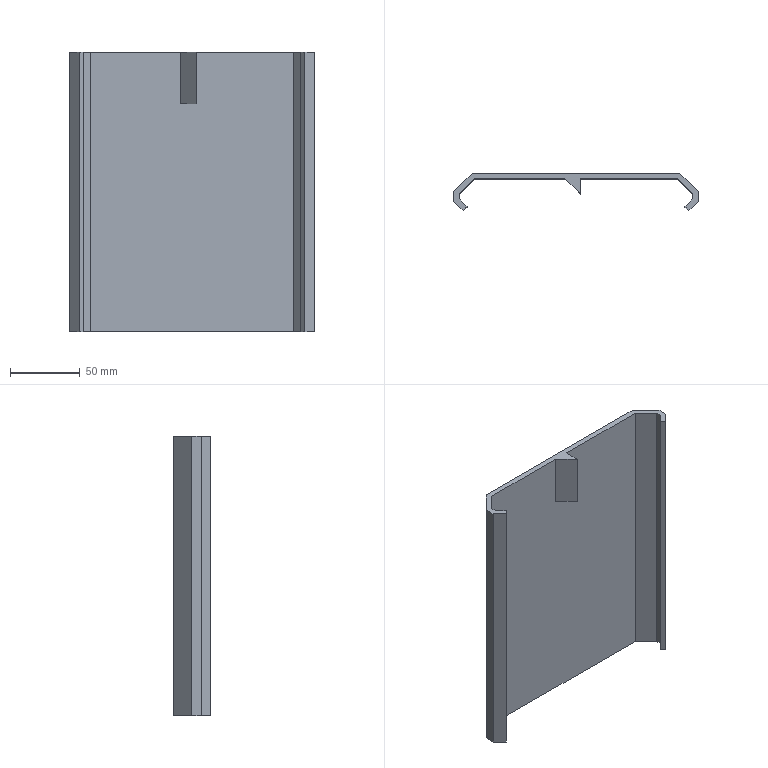Part | SolidWorks | features ExtruThin 1, ICE 1 | 1 solid | 21 faces | box 175 x 26.828 x 200 mm | volume 169317 mm3 | plane 21
STEP:
#1=CARTESIAN_POINT('',(83.5,37.5,0.));
#2=VERTEX_POINT('',#1);
#3=CARTESIAN_POINT('',(78.,32.,0.));
#4=VERTEX_POINT('',#3);
#5=CARTESIAN_POINT('',(83.5,37.5,0.));
#6=DIRECTION('',(-0.7071,-0.7071,0.));
#7=VECTOR('',#6,1000.);
#8=LINE('',#5,#7);
#9=EDGE_CURVE('',#2,#4,#8,.T.);
#10=ORIENTED_EDGE('',*,*,#9,.F.);
#11=CARTESIAN_POINT('',(83.5,37.5,-200.));
#12=VERTEX_POINT('',#11);
#13=CARTESIAN_POINT('',(83.5,37.5,-200.));
#14=DIRECTION('',(0.,0.,1.));
#15=VECTOR('',#14,1000.);
#16=LINE('',#13,#15);
#17=EDGE_CURVE('',#12,#2,#16,.T.);
#18=ORIENTED_EDGE('',*,*,#17,.F.);
#19=CARTESIAN_POINT('',(78.,32.,-200.));
#20=VERTEX_POINT('',#19);
#21=CARTESIAN_POINT('',(83.5,37.5,-200.));
#22=DIRECTION('',(-0.7071,-0.7071,0.));
#23=VECTOR('',#22,1000.);
#24=LINE('',#21,#23);
#25=EDGE_CURVE('',#12,#20,#24,.T.);
#26=ORIENTED_EDGE('',*,*,#25,.T.);
#27=CARTESIAN_POINT('',(78.,32.,-200.));
#28=DIRECTION('',(0.,0.,1.));
#29=VECTOR('',#28,1000.);
#30=LINE('',#27,#29);
#31=EDGE_CURVE('',#20,#4,#30,.T.);
#32=ORIENTED_EDGE('',*,*,#31,.T.);
#33=EDGE_LOOP('',(#10,#18,#26,#32));
#34=FACE_OUTER_BOUND('',#33,.T.);
#35=CARTESIAN_POINT('',(83.5,37.5,-200.));
#36=DIRECTION('',(-0.7071,0.7071,0.));
#37=DIRECTION('',(-0.7071,-0.7071,0.));
#38=AXIS2_PLACEMENT_3D('',#35,#36,#37);
#39=PLANE('',#38);
#40=ADVANCED_FACE('',(#34),#39,.T.);
#41=CARTESIAN_POINT('',(83.5,41.207,0.));
#42=VERTEX_POINT('',#41);
#43=CARTESIAN_POINT('',(83.5,41.207,0.));
#44=DIRECTION('',(0.,-1.,0.));
#45=VECTOR('',#44,1000.);
#46=LINE('',#43,#45);
#47=EDGE_CURVE('',#42,#2,#46,.T.);
#48=ORIENTED_EDGE('',*,*,#47,.F.);
#49=CARTESIAN_POINT('',(83.5,41.207,-200.));
#50=VERTEX_POINT('',#49);
#51=CARTESIAN_POINT('',(83.5,41.207,-200.));
#52=DIRECTION('',(0.,0.,1.));
#53=VECTOR('',#52,1000.);
#54=LINE('',#51,#53);
#55=EDGE_CURVE('',#50,#42,#54,.T.);
#56=ORIENTED_EDGE('',*,*,#55,.F.);
#57=CARTESIAN_POINT('',(83.5,41.207,-200.));
#58=DIRECTION('',(0.,-1.,0.));
#59=VECTOR('',#58,1000.);
#60=LINE('',#57,#59);
#61=EDGE_CURVE('',#50,#12,#60,.T.);
#62=ORIENTED_EDGE('',*,*,#61,.T.);
#63=ORIENTED_EDGE('',*,*,#17,.T.);
#64=EDGE_LOOP('',(#48,#56,#62,#63));
#65=FACE_OUTER_BOUND('',#64,.T.);
#66=CARTESIAN_POINT('',(83.5,41.207,-200.));
#67=DIRECTION('',(-1.,0.,0.));
#68=DIRECTION('',(0.,0.,1.));
#69=AXIS2_PLACEMENT_3D('',#66,#67,#68);
#70=PLANE('',#69);
#71=ADVANCED_FACE('',(#65),#70,.T.);
#72=CARTESIAN_POINT('',(72.707,52.,0.));
#73=VERTEX_POINT('',#72);
#74=CARTESIAN_POINT('',(72.707,52.,0.));
#75=DIRECTION('',(0.7071,-0.7071,0.));
#76=VECTOR('',#75,1000.);
#77=LINE('',#74,#76);
#78=EDGE_CURVE('',#73,#42,#77,.T.);
#79=ORIENTED_EDGE('',*,*,#78,.F.);
#80=CARTESIAN_POINT('',(72.707,52.,-200.));
#81=VERTEX_POINT('',#80);
#82=CARTESIAN_POINT('',(72.707,52.,-200.));
#83=DIRECTION('',(0.,0.,1.));
#84=VECTOR('',#83,1000.);
#85=LINE('',#82,#84);
#86=EDGE_CURVE('',#81,#73,#85,.T.);
#87=ORIENTED_EDGE('',*,*,#86,.F.);
#88=CARTESIAN_POINT('',(72.707,52.,-200.));
#89=DIRECTION('',(0.7071,-0.7071,0.));
#90=VECTOR('',#89,1000.);
#91=LINE('',#88,#90);
#92=EDGE_CURVE('',#81,#50,#91,.T.);
#93=ORIENTED_EDGE('',*,*,#92,.T.);
#94=ORIENTED_EDGE('',*,*,#55,.T.);
#95=EDGE_LOOP('',(#79,#87,#93,#94));
#96=FACE_OUTER_BOUND('',#95,.T.);
#97=CARTESIAN_POINT('',(72.707,52.,-200.));
#98=DIRECTION('',(-0.7071,-0.7071,0.));
#99=DIRECTION('',(0.7071,-0.7071,0.));
#100=AXIS2_PLACEMENT_3D('',#97,#98,#99);
#101=PLANE('',#100);
#102=ADVANCED_FACE('',(#96),#101,.T.);
#103=CARTESIAN_POINT('',(-7.99,52.,-37.));
#104=VERTEX_POINT('',#103);
#105=CARTESIAN_POINT('',(-7.99,52.,0.));
#106=VERTEX_POINT('',#105);
#107=CARTESIAN_POINT('',(-7.99,52.,-37.));
#108=DIRECTION('',(0.,0.,1.));
#109=VECTOR('',#108,1000.);
#110=LINE('',#107,#109);
#111=EDGE_CURVE('',#104,#106,#110,.T.);
#112=ORIENTED_EDGE('',*,*,#111,.T.);
#113=CARTESIAN_POINT('',(-72.707,52.,0.));
#114=VERTEX_POINT('',#113);
#115=CARTESIAN_POINT('',(72.707,52.,0.));
#116=DIRECTION('',(1.,0.,0.));
#117=VECTOR('',#116,1000.);
#118=LINE('',#115,#117);
#119=EDGE_CURVE('',#114,#106,#118,.T.);
#120=ORIENTED_EDGE('',*,*,#119,.F.);
#121=CARTESIAN_POINT('',(-72.707,52.,-200.));
#122=VERTEX_POINT('',#121);
#123=CARTESIAN_POINT('',(-72.707,52.,-200.));
#124=DIRECTION('',(0.,0.,1.));
#125=VECTOR('',#124,1000.);
#126=LINE('',#123,#125);
#127=EDGE_CURVE('',#122,#114,#126,.T.);
#128=ORIENTED_EDGE('',*,*,#127,.F.);
#129=CARTESIAN_POINT('',(72.707,52.,-200.));
#130=DIRECTION('',(1.,0.,0.));
#131=VECTOR('',#130,1000.);
#132=LINE('',#129,#131);
#133=EDGE_CURVE('',#122,#81,#132,.T.);
#134=ORIENTED_EDGE('',*,*,#133,.T.);
#135=ORIENTED_EDGE('',*,*,#86,.T.);
#136=CARTESIAN_POINT('',(3.,52.,0.));
#137=VERTEX_POINT('',#136);
#138=CARTESIAN_POINT('',(72.707,52.,0.));
#139=DIRECTION('',(1.,0.,0.));
#140=VECTOR('',#139,1000.);
#141=LINE('',#138,#140);
#142=EDGE_CURVE('',#137,#73,#141,.T.);
#143=ORIENTED_EDGE('',*,*,#142,.F.);
#144=CARTESIAN_POINT('',(3.,52.,-37.));
#145=VERTEX_POINT('',#144);
#146=CARTESIAN_POINT('',(3.,52.,-37.));
#147=DIRECTION('',(0.,0.,1.));
#148=VECTOR('',#147,1000.);
#149=LINE('',#146,#148);
#150=EDGE_CURVE('',#145,#137,#149,.T.);
#151=ORIENTED_EDGE('',*,*,#150,.F.);
#152=CARTESIAN_POINT('',(-7.99,52.,-37.));
#153=DIRECTION('',(-1.,0.,0.));
#154=VECTOR('',#153,1000.);
#155=LINE('',#152,#154);
#156=EDGE_CURVE('',#145,#104,#155,.T.);
#157=ORIENTED_EDGE('',*,*,#156,.T.);
#158=EDGE_LOOP('',(#112,#120,#128,#134,#135,#143,#151,#157));
#159=FACE_OUTER_BOUND('',#158,.T.);
#160=CARTESIAN_POINT('',(72.707,52.,-200.));
#161=DIRECTION('',(0.,-1.,0.));
#162=DIRECTION('',(0.,0.,-1.));
#163=AXIS2_PLACEMENT_3D('',#160,#161,#162);
#164=PLANE('',#163);
#165=ADVANCED_FACE('',(#159),#164,.T.);
#166=CARTESIAN_POINT('',(-83.5,41.207,0.));
#167=VERTEX_POINT('',#166);
#168=CARTESIAN_POINT('',(-72.707,52.,0.));
#169=DIRECTION('',(0.7071,0.7071,0.));
#170=VECTOR('',#169,1000.);
#171=LINE('',#168,#170);
#172=EDGE_CURVE('',#167,#114,#171,.T.);
#173=ORIENTED_EDGE('',*,*,#172,.F.);
#174=CARTESIAN_POINT('',(-83.5,41.207,-200.));
#175=VERTEX_POINT('',#174);
#176=CARTESIAN_POINT('',(-83.5,41.207,-200.));
#177=DIRECTION('',(0.,0.,1.));
#178=VECTOR('',#177,1000.);
#179=LINE('',#176,#178);
#180=EDGE_CURVE('',#175,#167,#179,.T.);
#181=ORIENTED_EDGE('',*,*,#180,.F.);
#182=CARTESIAN_POINT('',(-72.707,52.,-200.));
#183=DIRECTION('',(0.7071,0.7071,0.));
#184=VECTOR('',#183,1000.);
#185=LINE('',#182,#184);
#186=EDGE_CURVE('',#175,#122,#185,.T.);
#187=ORIENTED_EDGE('',*,*,#186,.T.);
#188=ORIENTED_EDGE('',*,*,#127,.T.);
#189=EDGE_LOOP('',(#173,#181,#187,#188));
#190=FACE_OUTER_BOUND('',#189,.T.);
#191=CARTESIAN_POINT('',(-72.707,52.,-200.));
#192=DIRECTION('',(0.7071,-0.7071,0.));
#193=DIRECTION('',(0.7071,0.7071,0.));
#194=AXIS2_PLACEMENT_3D('',#191,#192,#193);
#195=PLANE('',#194);
#196=ADVANCED_FACE('',(#190),#195,.T.);
#197=CARTESIAN_POINT('',(-83.5,37.5,0.));
#198=VERTEX_POINT('',#197);
#199=CARTESIAN_POINT('',(-83.5,41.207,0.));
#200=DIRECTION('',(0.,1.,0.));
#201=VECTOR('',#200,1000.);
#202=LINE('',#199,#201);
#203=EDGE_CURVE('',#198,#167,#202,.T.);
#204=ORIENTED_EDGE('',*,*,#203,.F.);
#205=CARTESIAN_POINT('',(-83.5,37.5,-200.));
#206=VERTEX_POINT('',#205);
#207=CARTESIAN_POINT('',(-83.5,37.5,-200.));
#208=DIRECTION('',(0.,0.,1.));
#209=VECTOR('',#208,1000.);
#210=LINE('',#207,#209);
#211=EDGE_CURVE('',#206,#198,#210,.T.);
#212=ORIENTED_EDGE('',*,*,#211,.F.);
#213=CARTESIAN_POINT('',(-83.5,41.207,-200.));
#214=DIRECTION('',(0.,1.,0.));
#215=VECTOR('',#214,1000.);
#216=LINE('',#213,#215);
#217=EDGE_CURVE('',#206,#175,#216,.T.);
#218=ORIENTED_EDGE('',*,*,#217,.T.);
#219=ORIENTED_EDGE('',*,*,#180,.T.);
#220=EDGE_LOOP('',(#204,#212,#218,#219));
#221=FACE_OUTER_BOUND('',#220,.T.);
#222=CARTESIAN_POINT('',(-83.5,41.207,-200.));
#223=DIRECTION('',(1.,0.,0.));
#224=DIRECTION('',(0.,0.,-1.));
#225=AXIS2_PLACEMENT_3D('',#222,#223,#224);
#226=PLANE('',#225);
#227=ADVANCED_FACE('',(#221),#226,.T.);
#228=CARTESIAN_POINT('',(-78.,32.,0.));
#229=VERTEX_POINT('',#228);
#230=CARTESIAN_POINT('',(-83.5,37.5,0.));
#231=DIRECTION('',(-0.7071,0.7071,0.));
#232=VECTOR('',#231,1000.);
#233=LINE('',#230,#232);
#234=EDGE_CURVE('',#229,#198,#233,.T.);
#235=ORIENTED_EDGE('',*,*,#234,.F.);
#236=CARTESIAN_POINT('',(-78.,32.,-200.));
#237=VERTEX_POINT('',#236);
#238=CARTESIAN_POINT('',(-78.,32.,-200.));
#239=DIRECTION('',(0.,0.,1.));
#240=VECTOR('',#239,1000.);
#241=LINE('',#238,#240);
#242=EDGE_CURVE('',#237,#229,#241,.T.);
#243=ORIENTED_EDGE('',*,*,#242,.F.);
#244=CARTESIAN_POINT('',(-83.5,37.5,-200.));
#245=DIRECTION('',(-0.7071,0.7071,0.));
#246=VECTOR('',#245,1000.);
#247=LINE('',#244,#246);
#248=EDGE_CURVE('',#237,#206,#247,.T.);
#249=ORIENTED_EDGE('',*,*,#248,.T.);
#250=ORIENTED_EDGE('',*,*,#211,.T.);
#251=EDGE_LOOP('',(#235,#243,#249,#250));
#252=FACE_OUTER_BOUND('',#251,.T.);
#253=CARTESIAN_POINT('',(-83.5,37.5,-200.));
#254=DIRECTION('',(0.7071,0.7071,0.));
#255=DIRECTION('',(-0.7071,0.7071,0.));
#256=AXIS2_PLACEMENT_3D('',#253,#254,#255);
#257=PLANE('',#256);
#258=ADVANCED_FACE('',(#252),#257,.T.);
#259=CARTESIAN_POINT('',(-80.828,29.172,0.));
#260=VERTEX_POINT('',#259);
#261=CARTESIAN_POINT('',(-78.,32.,0.));
#262=DIRECTION('',(-0.7071,-0.7071,0.));
#263=VECTOR('',#262,1000.);
#264=LINE('',#261,#263);
#265=EDGE_CURVE('',#229,#260,#264,.T.);
#266=ORIENTED_EDGE('',*,*,#265,.T.);
#267=CARTESIAN_POINT('',(-80.828,29.172,-200.));
#268=VERTEX_POINT('',#267);
#269=CARTESIAN_POINT('',(-80.828,29.172,-200.));
#270=DIRECTION('',(0.,0.,1.));
#271=VECTOR('',#270,1000.);
#272=LINE('',#269,#271);
#273=EDGE_CURVE('',#268,#260,#272,.T.);
#274=ORIENTED_EDGE('',*,*,#273,.F.);
#275=CARTESIAN_POINT('',(-78.,32.,-200.));
#276=DIRECTION('',(-0.7071,-0.7071,0.));
#277=VECTOR('',#276,1000.);
#278=LINE('',#275,#277);
#279=EDGE_CURVE('',#237,#268,#278,.T.);
#280=ORIENTED_EDGE('',*,*,#279,.F.);
#281=ORIENTED_EDGE('',*,*,#242,.T.);
#282=EDGE_LOOP('',(#266,#274,#280,#281));
#283=FACE_OUTER_BOUND('',#282,.T.);
#284=CARTESIAN_POINT('',(-78.,32.,-200.));
#285=DIRECTION('',(-0.7071,0.7071,0.));
#286=DIRECTION('',(-0.7071,-0.7071,0.));
#287=AXIS2_PLACEMENT_3D('',#284,#285,#286);
#288=PLANE('',#287);
#289=ADVANCED_FACE('',(#283),#288,.F.);
#290=CARTESIAN_POINT('',(-87.5,35.843,0.));
#291=VERTEX_POINT('',#290);
#292=CARTESIAN_POINT('',(-86.328,34.672,0.));
#293=DIRECTION('',(-0.7071,0.7071,0.));
#294=VECTOR('',#293,1000.);
#295=LINE('',#292,#294);
#296=EDGE_CURVE('',#260,#291,#295,.T.);
#297=ORIENTED_EDGE('',*,*,#296,.T.);
#298=CARTESIAN_POINT('',(-87.5,35.843,-200.));
#299=VERTEX_POINT('',#298);
#300=CARTESIAN_POINT('',(-87.5,35.843,-200.));
#301=DIRECTION('',(0.,0.,1.));
#302=VECTOR('',#301,1000.);
#303=LINE('',#300,#302);
#304=EDGE_CURVE('',#299,#291,#303,.T.);
#305=ORIENTED_EDGE('',*,*,#304,.F.);
#306=CARTESIAN_POINT('',(-86.328,34.672,-200.));
#307=DIRECTION('',(-0.7071,0.7071,0.));
#308=VECTOR('',#307,1000.);
#309=LINE('',#306,#308);
#310=EDGE_CURVE('',#268,#299,#309,.T.);
#311=ORIENTED_EDGE('',*,*,#310,.F.);
#312=ORIENTED_EDGE('',*,*,#273,.T.);
#313=EDGE_LOOP('',(#297,#305,#311,#312));
#314=FACE_OUTER_BOUND('',#313,.T.);
#315=CARTESIAN_POINT('',(-86.328,34.672,-200.));
#316=DIRECTION('',(0.7071,0.7071,0.));
#317=DIRECTION('',(-0.7071,0.7071,0.));
#318=AXIS2_PLACEMENT_3D('',#315,#316,#317);
#319=PLANE('',#318);
#320=ADVANCED_FACE('',(#314),#319,.F.);
#321=CARTESIAN_POINT('',(-87.5,42.864,0.));
#322=VERTEX_POINT('',#321);
#323=CARTESIAN_POINT('',(-87.5,41.207,0.));
#324=DIRECTION('',(0.,1.,0.));
#325=VECTOR('',#324,1000.);
#326=LINE('',#323,#325);
#327=EDGE_CURVE('',#291,#322,#326,.T.);
#328=ORIENTED_EDGE('',*,*,#327,.T.);
#329=CARTESIAN_POINT('',(-87.5,42.864,-200.));
#330=VERTEX_POINT('',#329);
#331=CARTESIAN_POINT('',(-87.5,42.864,-200.));
#332=DIRECTION('',(0.,0.,1.));
#333=VECTOR('',#332,1000.);
#334=LINE('',#331,#333);
#335=EDGE_CURVE('',#330,#322,#334,.T.);
#336=ORIENTED_EDGE('',*,*,#335,.F.);
#337=CARTESIAN_POINT('',(-87.5,41.207,-200.));
#338=DIRECTION('',(0.,1.,0.));
#339=VECTOR('',#338,1000.);
#340=LINE('',#337,#339);
#341=EDGE_CURVE('',#299,#330,#340,.T.);
#342=ORIENTED_EDGE('',*,*,#341,.F.);
#343=ORIENTED_EDGE('',*,*,#304,.T.);
#344=EDGE_LOOP('',(#328,#336,#342,#343));
#345=FACE_OUTER_BOUND('',#344,.T.);
#346=CARTESIAN_POINT('',(-87.5,41.207,-200.));
#347=DIRECTION('',(1.,0.,0.));
#348=DIRECTION('',(0.,0.,-1.));
#349=AXIS2_PLACEMENT_3D('',#346,#347,#348);
#350=PLANE('',#349);
#351=ADVANCED_FACE('',(#345),#350,.F.);
#352=CARTESIAN_POINT('',(-74.364,56.,0.));
#353=VERTEX_POINT('',#352);
#354=CARTESIAN_POINT('',(-75.536,54.828,0.));
#355=DIRECTION('',(0.7071,0.7071,0.));
#356=VECTOR('',#355,1000.);
#357=LINE('',#354,#356);
#358=EDGE_CURVE('',#322,#353,#357,.T.);
#359=ORIENTED_EDGE('',*,*,#358,.T.);
#360=CARTESIAN_POINT('',(-74.364,56.,-200.));
#361=VERTEX_POINT('',#360);
#362=CARTESIAN_POINT('',(-74.364,56.,-200.));
#363=DIRECTION('',(0.,0.,1.));
#364=VECTOR('',#363,1000.);
#365=LINE('',#362,#364);
#366=EDGE_CURVE('',#361,#353,#365,.T.);
#367=ORIENTED_EDGE('',*,*,#366,.F.);
#368=CARTESIAN_POINT('',(-75.536,54.828,-200.));
#369=DIRECTION('',(0.7071,0.7071,0.));
#370=VECTOR('',#369,1000.);
#371=LINE('',#368,#370);
#372=EDGE_CURVE('',#330,#361,#371,.T.);
#373=ORIENTED_EDGE('',*,*,#372,.F.);
#374=ORIENTED_EDGE('',*,*,#335,.T.);
#375=EDGE_LOOP('',(#359,#367,#373,#374));
#376=FACE_OUTER_BOUND('',#375,.T.);
#377=CARTESIAN_POINT('',(-75.536,54.828,-200.));
#378=DIRECTION('',(0.7071,-0.7071,0.));
#379=DIRECTION('',(0.7071,0.7071,0.));
#380=AXIS2_PLACEMENT_3D('',#377,#378,#379);
#381=PLANE('',#380);
#382=ADVANCED_FACE('',(#376),#381,.F.);
#383=CARTESIAN_POINT('',(74.364,56.,0.));
#384=VERTEX_POINT('',#383);
#385=CARTESIAN_POINT('',(72.707,56.,0.));
#386=DIRECTION('',(1.,0.,0.));
#387=VECTOR('',#386,1000.);
#388=LINE('',#385,#387);
#389=EDGE_CURVE('',#353,#384,#388,.T.);
#390=ORIENTED_EDGE('',*,*,#389,.T.);
#391=CARTESIAN_POINT('',(74.364,56.,-200.));
#392=VERTEX_POINT('',#391);
#393=CARTESIAN_POINT('',(74.364,56.,-200.));
#394=DIRECTION('',(0.,0.,1.));
#395=VECTOR('',#394,1000.);
#396=LINE('',#393,#395);
#397=EDGE_CURVE('',#392,#384,#396,.T.);
#398=ORIENTED_EDGE('',*,*,#397,.F.);
#399=CARTESIAN_POINT('',(72.707,56.,-200.));
#400=DIRECTION('',(1.,0.,0.));
#401=VECTOR('',#400,1000.);
#402=LINE('',#399,#401);
#403=EDGE_CURVE('',#361,#392,#402,.T.);
#404=ORIENTED_EDGE('',*,*,#403,.F.);
#405=ORIENTED_EDGE('',*,*,#366,.T.);
#406=EDGE_LOOP('',(#390,#398,#404,#405));
#407=FACE_OUTER_BOUND('',#406,.T.);
#408=CARTESIAN_POINT('',(72.707,56.,-200.));
#409=DIRECTION('',(0.,-1.,0.));
#410=DIRECTION('',(0.,0.,-1.));
#411=AXIS2_PLACEMENT_3D('',#408,#409,#410);
#412=PLANE('',#411);
#413=ADVANCED_FACE('',(#407),#412,.F.);
#414=CARTESIAN_POINT('',(87.5,42.864,0.));
#415=VERTEX_POINT('',#414);
#416=CARTESIAN_POINT('',(75.536,54.828,0.));
#417=DIRECTION('',(0.7071,-0.7071,0.));
#418=VECTOR('',#417,1000.);
#419=LINE('',#416,#418);
#420=EDGE_CURVE('',#384,#415,#419,.T.);
#421=ORIENTED_EDGE('',*,*,#420,.T.);
#422=CARTESIAN_POINT('',(87.5,42.864,-200.));
#423=VERTEX_POINT('',#422);
#424=CARTESIAN_POINT('',(87.5,42.864,-200.));
#425=DIRECTION('',(0.,0.,1.));
#426=VECTOR('',#425,1000.);
#427=LINE('',#424,#426);
#428=EDGE_CURVE('',#423,#415,#427,.T.);
#429=ORIENTED_EDGE('',*,*,#428,.F.);
#430=CARTESIAN_POINT('',(75.536,54.828,-200.));
#431=DIRECTION('',(0.7071,-0.7071,0.));
#432=VECTOR('',#431,1000.);
#433=LINE('',#430,#432);
#434=EDGE_CURVE('',#392,#423,#433,.T.);
#435=ORIENTED_EDGE('',*,*,#434,.F.);
#436=ORIENTED_EDGE('',*,*,#397,.T.);
#437=EDGE_LOOP('',(#421,#429,#435,#436));
#438=FACE_OUTER_BOUND('',#437,.T.);
#439=CARTESIAN_POINT('',(75.536,54.828,-200.));
#440=DIRECTION('',(-0.7071,-0.7071,0.));
#441=DIRECTION('',(0.7071,-0.7071,0.));
#442=AXIS2_PLACEMENT_3D('',#439,#440,#441);
#443=PLANE('',#442);
#444=ADVANCED_FACE('',(#438),#443,.F.);
#445=CARTESIAN_POINT('',(87.5,35.843,0.));
#446=VERTEX_POINT('',#445);
#447=CARTESIAN_POINT('',(87.5,41.207,0.));
#448=DIRECTION('',(0.,-1.,0.));
#449=VECTOR('',#448,1000.);
#450=LINE('',#447,#449);
#451=EDGE_CURVE('',#415,#446,#450,.T.);
#452=ORIENTED_EDGE('',*,*,#451,.T.);
#453=CARTESIAN_POINT('',(87.5,35.843,-200.));
#454=VERTEX_POINT('',#453);
#455=CARTESIAN_POINT('',(87.5,35.843,-200.));
#456=DIRECTION('',(0.,0.,1.));
#457=VECTOR('',#456,1000.);
#458=LINE('',#455,#457);
#459=EDGE_CURVE('',#454,#446,#458,.T.);
#460=ORIENTED_EDGE('',*,*,#459,.F.);
#461=CARTESIAN_POINT('',(87.5,41.207,-200.));
#462=DIRECTION('',(0.,-1.,0.));
#463=VECTOR('',#462,1000.);
#464=LINE('',#461,#463);
#465=EDGE_CURVE('',#423,#454,#464,.T.);
#466=ORIENTED_EDGE('',*,*,#465,.F.);
#467=ORIENTED_EDGE('',*,*,#428,.T.);
#468=EDGE_LOOP('',(#452,#460,#466,#467));
#469=FACE_OUTER_BOUND('',#468,.T.);
#470=CARTESIAN_POINT('',(87.5,41.207,-200.));
#471=DIRECTION('',(-1.,0.,0.));
#472=DIRECTION('',(0.,0.,1.));
#473=AXIS2_PLACEMENT_3D('',#470,#471,#472);
#474=PLANE('',#473);
#475=ADVANCED_FACE('',(#469),#474,.F.);
#476=CARTESIAN_POINT('',(80.828,29.172,0.));
#477=VERTEX_POINT('',#476);
#478=CARTESIAN_POINT('',(86.328,34.672,0.));
#479=DIRECTION('',(-0.7071,-0.7071,0.));
#480=VECTOR('',#479,1000.);
#481=LINE('',#478,#480);
#482=EDGE_CURVE('',#446,#477,#481,.T.);
#483=ORIENTED_EDGE('',*,*,#482,.T.);
#484=CARTESIAN_POINT('',(80.828,29.172,-200.));
#485=VERTEX_POINT('',#484);
#486=CARTESIAN_POINT('',(80.828,29.172,-200.));
#487=DIRECTION('',(0.,0.,1.));
#488=VECTOR('',#487,1000.);
#489=LINE('',#486,#488);
#490=EDGE_CURVE('',#485,#477,#489,.T.);
#491=ORIENTED_EDGE('',*,*,#490,.F.);
#492=CARTESIAN_POINT('',(86.328,34.672,-200.));
#493=DIRECTION('',(-0.7071,-0.7071,0.));
#494=VECTOR('',#493,1000.);
#495=LINE('',#492,#494);
#496=EDGE_CURVE('',#454,#485,#495,.T.);
#497=ORIENTED_EDGE('',*,*,#496,.F.);
#498=ORIENTED_EDGE('',*,*,#459,.T.);
#499=EDGE_LOOP('',(#483,#491,#497,#498));
#500=FACE_OUTER_BOUND('',#499,.T.);
#501=CARTESIAN_POINT('',(86.328,34.672,-200.));
#502=DIRECTION('',(-0.7071,0.7071,0.));
#503=DIRECTION('',(-0.7071,-0.7071,0.));
#504=AXIS2_PLACEMENT_3D('',#501,#502,#503);
#505=PLANE('',#504);
#506=ADVANCED_FACE('',(#500),#505,.F.);
#507=CARTESIAN_POINT('',(80.828,29.172,0.));
#508=DIRECTION('',(-0.7071,0.7071,0.));
#509=VECTOR('',#508,1000.);
#510=LINE('',#507,#509);
#511=EDGE_CURVE('',#477,#4,#510,.T.);
#512=ORIENTED_EDGE('',*,*,#511,.T.);
#513=ORIENTED_EDGE('',*,*,#31,.F.);
#514=CARTESIAN_POINT('',(80.828,29.172,-200.));
#515=DIRECTION('',(-0.7071,0.7071,0.));
#516=VECTOR('',#515,1000.);
#517=LINE('',#514,#516);
#518=EDGE_CURVE('',#485,#20,#517,.T.);
#519=ORIENTED_EDGE('',*,*,#518,.F.);
#520=ORIENTED_EDGE('',*,*,#490,.T.);
#521=EDGE_LOOP('',(#512,#513,#519,#520));
#522=FACE_OUTER_BOUND('',#521,.T.);
#523=CARTESIAN_POINT('',(80.828,29.172,-200.));
#524=DIRECTION('',(0.7071,0.7071,0.));
#525=DIRECTION('',(-0.7071,0.7071,0.));
#526=AXIS2_PLACEMENT_3D('',#523,#524,#525);
#527=PLANE('',#526);
#528=ADVANCED_FACE('',(#522),#527,.F.);
#529=ORIENTED_EDGE('',*,*,#25,.F.);
#530=ORIENTED_EDGE('',*,*,#61,.F.);
#531=ORIENTED_EDGE('',*,*,#92,.F.);
#532=ORIENTED_EDGE('',*,*,#133,.F.);
#533=ORIENTED_EDGE('',*,*,#186,.F.);
#534=ORIENTED_EDGE('',*,*,#217,.F.);
#535=ORIENTED_EDGE('',*,*,#248,.F.);
#536=ORIENTED_EDGE('',*,*,#279,.T.);
#537=ORIENTED_EDGE('',*,*,#310,.T.);
#538=ORIENTED_EDGE('',*,*,#341,.T.);
#539=ORIENTED_EDGE('',*,*,#372,.T.);
#540=ORIENTED_EDGE('',*,*,#403,.T.);
#541=ORIENTED_EDGE('',*,*,#434,.T.);
#542=ORIENTED_EDGE('',*,*,#465,.T.);
#543=ORIENTED_EDGE('',*,*,#496,.T.);
#544=ORIENTED_EDGE('',*,*,#518,.T.);
#545=EDGE_LOOP('',(#529,#530,#531,#532,#533,#534,#535,#536,#537,#538,#539,#540,#541,#542,#543,#544));
#546=FACE_OUTER_BOUND('',#545,.T.);
#547=CARTESIAN_POINT('',(0.,0.,-200.));
#548=DIRECTION('',(0.,0.,-1.));
#549=DIRECTION('',(-1.,0.,0.));
#550=AXIS2_PLACEMENT_3D('',#547,#548,#549);
#551=PLANE('',#550);
#552=ADVANCED_FACE('',(#546),#551,.T.);
#553=ORIENTED_EDGE('',*,*,#9,.T.);
#554=ORIENTED_EDGE('',*,*,#511,.F.);
#555=ORIENTED_EDGE('',*,*,#482,.F.);
#556=ORIENTED_EDGE('',*,*,#451,.F.);
#557=ORIENTED_EDGE('',*,*,#420,.F.);
#558=ORIENTED_EDGE('',*,*,#389,.F.);
#559=ORIENTED_EDGE('',*,*,#358,.F.);
#560=ORIENTED_EDGE('',*,*,#327,.F.);
#561=ORIENTED_EDGE('',*,*,#296,.F.);
#562=ORIENTED_EDGE('',*,*,#265,.F.);
#563=ORIENTED_EDGE('',*,*,#234,.T.);
#564=ORIENTED_EDGE('',*,*,#203,.T.);
#565=ORIENTED_EDGE('',*,*,#172,.T.);
#566=ORIENTED_EDGE('',*,*,#119,.T.);
#567=CARTESIAN_POINT('',(3.,41.01,0.));
#568=VERTEX_POINT('',#567);
#569=CARTESIAN_POINT('',(3.,41.01,0.));
#570=DIRECTION('',(0.7071,-0.7071,0.));
#571=VECTOR('',#570,1000.);
#572=LINE('',#569,#571);
#573=EDGE_CURVE('',#106,#568,#572,.T.);
#574=ORIENTED_EDGE('',*,*,#573,.T.);
#575=CARTESIAN_POINT('',(3.,52.,0.));
#576=DIRECTION('',(0.,1.,0.));
#577=VECTOR('',#576,1000.);
#578=LINE('',#575,#577);
#579=EDGE_CURVE('',#568,#137,#578,.T.);
#580=ORIENTED_EDGE('',*,*,#579,.T.);
#581=ORIENTED_EDGE('',*,*,#142,.T.);
#582=ORIENTED_EDGE('',*,*,#78,.T.);
#583=ORIENTED_EDGE('',*,*,#47,.T.);
#584=EDGE_LOOP('',(#553,#554,#555,#556,#557,#558,#559,#560,#561,#562,#563,#564,#565,#566,#574,#580,#581,#582,#583));
#585=FACE_OUTER_BOUND('',#584,.T.);
#586=CARTESIAN_POINT('',(0.,0.,0.));
#587=DIRECTION('',(0.,0.,-1.));
#588=DIRECTION('',(-1.,0.,0.));
#589=AXIS2_PLACEMENT_3D('',#586,#587,#588);
#590=PLANE('',#589);
#591=ADVANCED_FACE('',(#585),#590,.F.);
#592=ORIENTED_EDGE('',*,*,#573,.F.);
#593=ORIENTED_EDGE('',*,*,#111,.F.);
#594=CARTESIAN_POINT('',(3.,41.01,-37.));
#595=VERTEX_POINT('',#594);
#596=CARTESIAN_POINT('',(3.,41.01,-37.));
#597=DIRECTION('',(0.7071,-0.7071,0.));
#598=VECTOR('',#597,1000.);
#599=LINE('',#596,#598);
#600=EDGE_CURVE('',#104,#595,#599,.T.);
#601=ORIENTED_EDGE('',*,*,#600,.T.);
#602=CARTESIAN_POINT('',(3.,41.01,-37.));
#603=DIRECTION('',(0.,0.,1.));
#604=VECTOR('',#603,1000.);
#605=LINE('',#602,#604);
#606=EDGE_CURVE('',#595,#568,#605,.T.);
#607=ORIENTED_EDGE('',*,*,#606,.T.);
#608=EDGE_LOOP('',(#592,#593,#601,#607));
#609=FACE_OUTER_BOUND('',#608,.T.);
#610=CARTESIAN_POINT('',(3.,41.01,-37.));
#611=DIRECTION('',(-0.7071,-0.7071,0.));
#612=DIRECTION('',(0.7071,-0.7071,0.));
#613=AXIS2_PLACEMENT_3D('',#610,#611,#612);
#614=PLANE('',#613);
#615=ADVANCED_FACE('',(#609),#614,.T.);
#616=ORIENTED_EDGE('',*,*,#579,.F.);
#617=ORIENTED_EDGE('',*,*,#606,.F.);
#618=CARTESIAN_POINT('',(3.,52.,-37.));
#619=DIRECTION('',(0.,1.,0.));
#620=VECTOR('',#619,1000.);
#621=LINE('',#618,#620);
#622=EDGE_CURVE('',#595,#145,#621,.T.);
#623=ORIENTED_EDGE('',*,*,#622,.T.);
#624=ORIENTED_EDGE('',*,*,#150,.T.);
#625=EDGE_LOOP('',(#616,#617,#623,#624));
#626=FACE_OUTER_BOUND('',#625,.T.);
#627=CARTESIAN_POINT('',(3.,52.,-37.));
#628=DIRECTION('',(1.,0.,0.));
#629=DIRECTION('',(0.,1.,0.));
#630=AXIS2_PLACEMENT_3D('',#627,#628,#629);
#631=PLANE('',#630);
#632=ADVANCED_FACE('',(#626),#631,.T.);
#633=ORIENTED_EDGE('',*,*,#600,.F.);
#634=ORIENTED_EDGE('',*,*,#156,.F.);
#635=ORIENTED_EDGE('',*,*,#622,.F.);
#636=EDGE_LOOP('',(#633,#634,#635));
#637=FACE_OUTER_BOUND('',#636,.T.);
#638=CARTESIAN_POINT('',(0.,0.,-37.));
#639=DIRECTION('',(0.,0.,-1.));
#640=DIRECTION('',(-1.,0.,0.));
#641=AXIS2_PLACEMENT_3D('',#638,#639,#640);
#642=PLANE('',#641);
#643=ADVANCED_FACE('',(#637),#642,.T.);
#644=CLOSED_SHELL('',(#40,#71,#102,#165,#196,#227,#258,#289,#320,#351,#382,#413,#444,#475,#506,#528,#552,#591,#615,#632,#643));
#645=MANIFOLD_SOLID_BREP('',#644);
#646=CARTESIAN_POINT('',(0.,0.,0.));
#647=DIRECTION('',(0.,0.,1.));
#648=DIRECTION('',(1.,0.,0.));
#649=AXIS2_PLACEMENT_3D('',#646,#647,#648);
#650=(LENGTH_UNIT()NAMED_UNIT(*)SI_UNIT(.MILLI.,.METRE.));
#651=UNCERTAINTY_MEASURE_WITH_UNIT(LENGTH_MEASURE(0.00001),#650,'','');
#652=(NAMED_UNIT(*)PLANE_ANGLE_UNIT()SI_UNIT($,.RADIAN.));
#653=(NAMED_UNIT(*)SI_UNIT($,.STERADIAN.)SOLID_ANGLE_UNIT());
#654=(GEOMETRIC_REPRESENTATION_CONTEXT(3)GLOBAL_UNCERTAINTY_ASSIGNED_CONTEXT((#651))GLOBAL_UNIT_ASSIGNED_CONTEXT((#650,#652,#653))REPRESENTATION_CONTEXT('',''));
#655=ADVANCED_BREP_SHAPE_REPRESENTATION('',(#645,#649),#654);